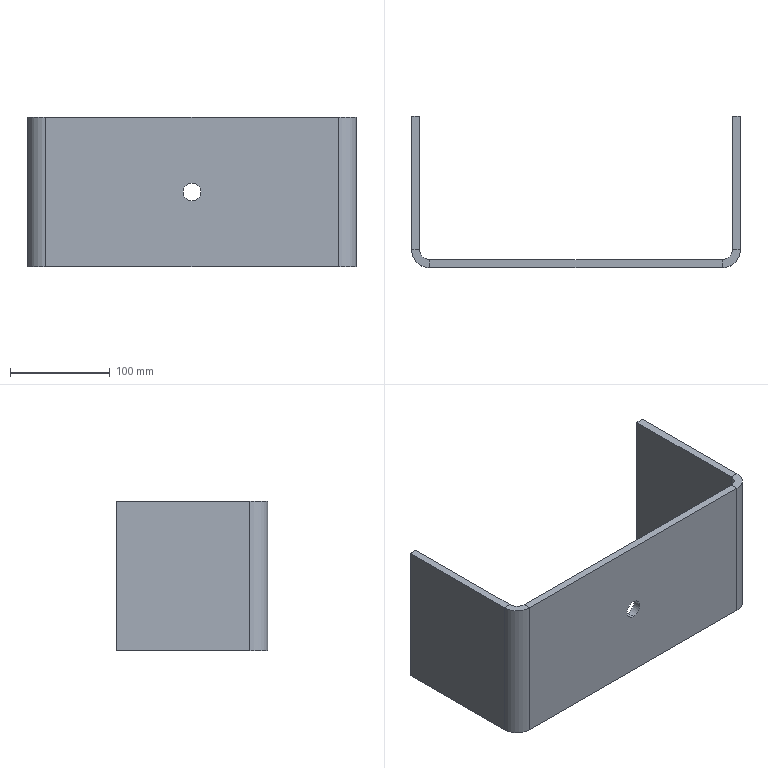Part | STEP file | A_SYL0380DJ1008_1_4-1_CHACHE_AS | 1 solid | 24 faces | box 330 x 152 x 150 mm | volume 725143 mm3 | plane 18 | cylinder 6 | commonest cylinder face diameters 18 x2 20 x2 36 x2
STEP:
#1=CARTESIAN_POINT('',(-165.,-62.,-75.));
#2=VERTEX_POINT('',#1);
#3=CARTESIAN_POINT('',(-165.,72.,-75.));
#4=VERTEX_POINT('',#3);
#5=CARTESIAN_POINT('',(-165.,-62.,-75.));
#6=DIRECTION('',(0.,1.,0.));
#7=VECTOR('',#6,1000.);
#8=LINE('',#5,#7);
#9=EDGE_CURVE('',#2,#4,#8,.T.);
#10=ORIENTED_EDGE('',*,*,#9,.F.);
#11=CARTESIAN_POINT('',(-165.,-62.,75.));
#12=VERTEX_POINT('',#11);
#13=CARTESIAN_POINT('',(-165.,-62.,75.));
#14=DIRECTION('',(0.,0.,-1.));
#15=VECTOR('',#14,1000.);
#16=LINE('',#13,#15);
#17=EDGE_CURVE('',#12,#2,#16,.T.);
#18=ORIENTED_EDGE('',*,*,#17,.F.);
#19=CARTESIAN_POINT('',(-165.,72.,75.));
#20=VERTEX_POINT('',#19);
#21=CARTESIAN_POINT('',(-165.,-62.,75.));
#22=DIRECTION('',(0.,1.,0.));
#23=VECTOR('',#22,1000.);
#24=LINE('',#21,#23);
#25=EDGE_CURVE('',#12,#20,#24,.T.);
#26=ORIENTED_EDGE('',*,*,#25,.T.);
#27=CARTESIAN_POINT('',(-165.,72.,75.));
#28=DIRECTION('',(0.,0.,-1.));
#29=VECTOR('',#28,1000.);
#30=LINE('',#27,#29);
#31=EDGE_CURVE('',#20,#4,#30,.T.);
#32=ORIENTED_EDGE('',*,*,#31,.T.);
#33=EDGE_LOOP('',(#10,#18,#26,#32));
#34=FACE_OUTER_BOUND('',#33,.T.);
#35=CARTESIAN_POINT('',(-165.,72.,-75.));
#36=DIRECTION('',(-1.,0.,0.));
#37=DIRECTION('',(0.,0.,1.));
#38=AXIS2_PLACEMENT_3D('',#35,#36,#37);
#39=PLANE('',#38);
#40=ADVANCED_FACE('',(#34),#39,.T.);
#41=CARTESIAN_POINT('',(165.,72.,75.));
#42=VERTEX_POINT('',#41);
#43=CARTESIAN_POINT('',(165.,-62.,75.));
#44=VERTEX_POINT('',#43);
#45=CARTESIAN_POINT('',(165.,72.,75.));
#46=DIRECTION('',(0.,-1.,0.));
#47=VECTOR('',#46,1000.);
#48=LINE('',#45,#47);
#49=EDGE_CURVE('',#42,#44,#48,.T.);
#50=ORIENTED_EDGE('',*,*,#49,.T.);
#51=CARTESIAN_POINT('',(165.,-62.,-75.));
#52=VERTEX_POINT('',#51);
#53=CARTESIAN_POINT('',(165.,-62.,-75.));
#54=DIRECTION('',(0.,0.,1.));
#55=VECTOR('',#54,1000.);
#56=LINE('',#53,#55);
#57=EDGE_CURVE('',#52,#44,#56,.T.);
#58=ORIENTED_EDGE('',*,*,#57,.F.);
#59=CARTESIAN_POINT('',(165.,72.,-75.));
#60=VERTEX_POINT('',#59);
#61=CARTESIAN_POINT('',(165.,72.,-75.));
#62=DIRECTION('',(0.,-1.,0.));
#63=VECTOR('',#62,1000.);
#64=LINE('',#61,#63);
#65=EDGE_CURVE('',#60,#52,#64,.T.);
#66=ORIENTED_EDGE('',*,*,#65,.F.);
#67=CARTESIAN_POINT('',(165.,72.,75.));
#68=DIRECTION('',(0.,0.,-1.));
#69=VECTOR('',#68,1000.);
#70=LINE('',#67,#69);
#71=EDGE_CURVE('',#42,#60,#70,.T.);
#72=ORIENTED_EDGE('',*,*,#71,.F.);
#73=EDGE_LOOP('',(#50,#58,#66,#72));
#74=FACE_OUTER_BOUND('',#73,.T.);
#75=CARTESIAN_POINT('',(165.,-80.,-75.));
#76=DIRECTION('',(1.,0.,0.));
#77=DIRECTION('',(0.,1.,0.));
#78=AXIS2_PLACEMENT_3D('',#75,#76,#77);
#79=PLANE('',#78);
#80=ADVANCED_FACE('',(#74),#79,.T.);
#81=CARTESIAN_POINT('',(147.,-80.,75.));
#82=VERTEX_POINT('',#81);
#83=CARTESIAN_POINT('',(147.,-62.,75.));
#84=DIRECTION('',(0.,0.,1.));
#85=DIRECTION('',(0.,-1.,0.));
#86=AXIS2_PLACEMENT_3D('',#83,#84,#85);
#87=CIRCLE('',#86,18.);
#88=EDGE_CURVE('',#82,#44,#87,.T.);
#89=ORIENTED_EDGE('',*,*,#88,.F.);
#90=CARTESIAN_POINT('',(147.,-80.,-75.));
#91=VERTEX_POINT('',#90);
#92=CARTESIAN_POINT('',(147.,-80.,75.));
#93=DIRECTION('',(0.,0.,-1.));
#94=VECTOR('',#93,1000.);
#95=LINE('',#92,#94);
#96=EDGE_CURVE('',#82,#91,#95,.T.);
#97=ORIENTED_EDGE('',*,*,#96,.T.);
#98=CARTESIAN_POINT('',(147.,-62.,-75.));
#99=DIRECTION('',(0.,0.,-1.));
#100=DIRECTION('',(1.,0.,0.));
#101=AXIS2_PLACEMENT_3D('',#98,#99,#100);
#102=CIRCLE('',#101,18.);
#103=EDGE_CURVE('',#52,#91,#102,.T.);
#104=ORIENTED_EDGE('',*,*,#103,.F.);
#105=ORIENTED_EDGE('',*,*,#57,.T.);
#106=EDGE_LOOP('',(#89,#97,#104,#105));
#107=FACE_OUTER_BOUND('',#106,.T.);
#108=CARTESIAN_POINT('',(147.,-62.,416.165));
#109=DIRECTION('',(0.,0.,-1.));
#110=DIRECTION('',(-1.,0.,0.));
#111=AXIS2_PLACEMENT_3D('',#108,#109,#110);
#112=CYLINDRICAL_SURFACE('',#111,18.);
#113=ADVANCED_FACE('',(#107),#112,.T.);
#114=CARTESIAN_POINT('',(0.,-80.,9.));
#115=VERTEX_POINT('',#114);
#116=CARTESIAN_POINT('',(0.,-72.,9.));
#117=VERTEX_POINT('',#116);
#118=CARTESIAN_POINT('',(0.,-80.,9.));
#119=DIRECTION('',(0.,1.,0.));
#120=VECTOR('',#119,1000.);
#121=LINE('',#118,#120);
#122=EDGE_CURVE('',#115,#117,#121,.T.);
#123=ORIENTED_EDGE('',*,*,#122,.F.);
#124=CARTESIAN_POINT('',(0.,-80.,-9.));
#125=VERTEX_POINT('',#124);
#126=CARTESIAN_POINT('',(0.,-80.,0.));
#127=DIRECTION('',(0.,1.,0.));
#128=DIRECTION('',(0.,0.,-1.));
#129=AXIS2_PLACEMENT_3D('',#126,#127,#128);
#130=CIRCLE('',#129,9.);
#131=EDGE_CURVE('',#125,#115,#130,.T.);
#132=ORIENTED_EDGE('',*,*,#131,.F.);
#133=CARTESIAN_POINT('',(0.,-72.,-9.));
#134=VERTEX_POINT('',#133);
#135=CARTESIAN_POINT('',(0.,-80.,-9.));
#136=DIRECTION('',(0.,1.,0.));
#137=VECTOR('',#136,1000.);
#138=LINE('',#135,#137);
#139=EDGE_CURVE('',#125,#134,#138,.T.);
#140=ORIENTED_EDGE('',*,*,#139,.T.);
#141=CARTESIAN_POINT('',(0.,-72.,0.));
#142=DIRECTION('',(0.,-1.,0.));
#143=DIRECTION('',(0.,0.,1.));
#144=AXIS2_PLACEMENT_3D('',#141,#142,#143);
#145=CIRCLE('',#144,9.);
#146=EDGE_CURVE('',#117,#134,#145,.T.);
#147=ORIENTED_EDGE('',*,*,#146,.F.);
#148=EDGE_LOOP('',(#123,#132,#140,#147));
#149=FACE_OUTER_BOUND('',#148,.T.);
#150=CARTESIAN_POINT('',(0.,-72.,0.));
#151=DIRECTION('',(0.,-1.,0.));
#152=DIRECTION('',(0.,0.,-1.));
#153=AXIS2_PLACEMENT_3D('',#150,#151,#152);
#154=CYLINDRICAL_SURFACE('',#153,9.);
#155=ADVANCED_FACE('',(#149),#154,.F.);
#156=CARTESIAN_POINT('',(0.,-72.,0.));
#157=DIRECTION('',(0.,-1.,0.));
#158=DIRECTION('',(0.,0.,-1.));
#159=AXIS2_PLACEMENT_3D('',#156,#157,#158);
#160=CIRCLE('',#159,9.);
#161=EDGE_CURVE('',#134,#117,#160,.T.);
#162=ORIENTED_EDGE('',*,*,#161,.F.);
#163=ORIENTED_EDGE('',*,*,#139,.F.);
#164=CARTESIAN_POINT('',(0.,-80.,0.));
#165=DIRECTION('',(0.,1.,0.));
#166=DIRECTION('',(0.,0.,1.));
#167=AXIS2_PLACEMENT_3D('',#164,#165,#166);
#168=CIRCLE('',#167,9.);
#169=EDGE_CURVE('',#115,#125,#168,.T.);
#170=ORIENTED_EDGE('',*,*,#169,.F.);
#171=ORIENTED_EDGE('',*,*,#122,.T.);
#172=EDGE_LOOP('',(#162,#163,#170,#171));
#173=FACE_OUTER_BOUND('',#172,.T.);
#174=CARTESIAN_POINT('',(0.,-72.,0.));
#175=DIRECTION('',(0.,-1.,0.));
#176=DIRECTION('',(0.,0.,-1.));
#177=AXIS2_PLACEMENT_3D('',#174,#175,#176);
#178=CYLINDRICAL_SURFACE('',#177,9.);
#179=ADVANCED_FACE('',(#173),#178,.F.);
#180=CARTESIAN_POINT('',(-157.,-62.,75.));
#181=VERTEX_POINT('',#180);
#182=CARTESIAN_POINT('',(-157.,72.,75.));
#183=VERTEX_POINT('',#182);
#184=CARTESIAN_POINT('',(-157.,-62.,75.));
#185=DIRECTION('',(0.,1.,0.));
#186=VECTOR('',#185,1000.);
#187=LINE('',#184,#186);
#188=EDGE_CURVE('',#181,#183,#187,.T.);
#189=ORIENTED_EDGE('',*,*,#188,.F.);
#190=CARTESIAN_POINT('',(-157.,-62.,-75.));
#191=VERTEX_POINT('',#190);
#192=CARTESIAN_POINT('',(-157.,-62.,-75.));
#193=DIRECTION('',(0.,0.,1.));
#194=VECTOR('',#193,1000.);
#195=LINE('',#192,#194);
#196=EDGE_CURVE('',#191,#181,#195,.T.);
#197=ORIENTED_EDGE('',*,*,#196,.F.);
#198=CARTESIAN_POINT('',(-157.,72.,-75.));
#199=VERTEX_POINT('',#198);
#200=CARTESIAN_POINT('',(-157.,-62.,-75.));
#201=DIRECTION('',(0.,1.,0.));
#202=VECTOR('',#201,1000.);
#203=LINE('',#200,#202);
#204=EDGE_CURVE('',#191,#199,#203,.T.);
#205=ORIENTED_EDGE('',*,*,#204,.T.);
#206=CARTESIAN_POINT('',(-157.,72.,75.));
#207=DIRECTION('',(0.,0.,-1.));
#208=VECTOR('',#207,1000.);
#209=LINE('',#206,#208);
#210=EDGE_CURVE('',#183,#199,#209,.T.);
#211=ORIENTED_EDGE('',*,*,#210,.F.);
#212=EDGE_LOOP('',(#189,#197,#205,#211));
#213=FACE_OUTER_BOUND('',#212,.T.);
#214=CARTESIAN_POINT('',(-157.,72.,-75.));
#215=DIRECTION('',(-1.,0.,0.));
#216=DIRECTION('',(0.,0.,1.));
#217=AXIS2_PLACEMENT_3D('',#214,#215,#216);
#218=PLANE('',#217);
#219=ADVANCED_FACE('',(#213),#218,.F.);
#220=CARTESIAN_POINT('',(-147.,-72.,-75.));
#221=VERTEX_POINT('',#220);
#222=CARTESIAN_POINT('',(-147.,-62.,-75.));
#223=DIRECTION('',(0.,0.,1.));
#224=DIRECTION('',(-1.,0.,0.));
#225=AXIS2_PLACEMENT_3D('',#222,#223,#224);
#226=CIRCLE('',#225,10.);
#227=EDGE_CURVE('',#191,#221,#226,.T.);
#228=ORIENTED_EDGE('',*,*,#227,.F.);
#229=ORIENTED_EDGE('',*,*,#196,.T.);
#230=CARTESIAN_POINT('',(-147.,-72.,75.));
#231=VERTEX_POINT('',#230);
#232=CARTESIAN_POINT('',(-147.,-62.,75.));
#233=DIRECTION('',(0.,0.,-1.));
#234=DIRECTION('',(0.,-1.,0.));
#235=AXIS2_PLACEMENT_3D('',#232,#233,#234);
#236=CIRCLE('',#235,10.);
#237=EDGE_CURVE('',#231,#181,#236,.T.);
#238=ORIENTED_EDGE('',*,*,#237,.F.);
#239=CARTESIAN_POINT('',(-147.,-72.,75.));
#240=DIRECTION('',(0.,0.,-1.));
#241=VECTOR('',#240,1000.);
#242=LINE('',#239,#241);
#243=EDGE_CURVE('',#231,#221,#242,.T.);
#244=ORIENTED_EDGE('',*,*,#243,.T.);
#245=EDGE_LOOP('',(#228,#229,#238,#244));
#246=FACE_OUTER_BOUND('',#245,.T.);
#247=CARTESIAN_POINT('',(-147.,-62.,416.165));
#248=DIRECTION('',(0.,0.,-1.));
#249=DIRECTION('',(-1.,0.,0.));
#250=AXIS2_PLACEMENT_3D('',#247,#248,#249);
#251=CYLINDRICAL_SURFACE('',#250,10.);
#252=ADVANCED_FACE('',(#246),#251,.F.);
#253=ORIENTED_EDGE('',*,*,#146,.T.);
#254=ORIENTED_EDGE('',*,*,#161,.T.);
#255=EDGE_LOOP('',(#253,#254));
#256=FACE_BOUND('',#255,.T.);
#257=CARTESIAN_POINT('',(147.,-72.,75.));
#258=VERTEX_POINT('',#257);
#259=CARTESIAN_POINT('',(147.,-72.,75.));
#260=DIRECTION('',(-1.,0.,0.));
#261=VECTOR('',#260,1000.);
#262=LINE('',#259,#261);
#263=EDGE_CURVE('',#258,#231,#262,.T.);
#264=ORIENTED_EDGE('',*,*,#263,.F.);
#265=CARTESIAN_POINT('',(147.,-72.,-75.));
#266=VERTEX_POINT('',#265);
#267=CARTESIAN_POINT('',(147.,-72.,-75.));
#268=DIRECTION('',(0.,0.,1.));
#269=VECTOR('',#268,1000.);
#270=LINE('',#267,#269);
#271=EDGE_CURVE('',#266,#258,#270,.T.);
#272=ORIENTED_EDGE('',*,*,#271,.F.);
#273=CARTESIAN_POINT('',(147.,-72.,-75.));
#274=DIRECTION('',(-1.,0.,0.));
#275=VECTOR('',#274,1000.);
#276=LINE('',#273,#275);
#277=EDGE_CURVE('',#266,#221,#276,.T.);
#278=ORIENTED_EDGE('',*,*,#277,.T.);
#279=ORIENTED_EDGE('',*,*,#243,.F.);
#280=EDGE_LOOP('',(#264,#272,#278,#279));
#281=FACE_OUTER_BOUND('',#280,.T.);
#282=CARTESIAN_POINT('',(-165.,-72.,-75.));
#283=DIRECTION('',(0.,-1.,0.));
#284=DIRECTION('',(0.,0.,-1.));
#285=AXIS2_PLACEMENT_3D('',#282,#283,#284);
#286=PLANE('',#285);
#287=ADVANCED_FACE('',(#256,#281),#286,.F.);
#288=CARTESIAN_POINT('',(157.,72.,-75.));
#289=VERTEX_POINT('',#288);
#290=CARTESIAN_POINT('',(157.,-62.,-75.));
#291=VERTEX_POINT('',#290);
#292=CARTESIAN_POINT('',(157.,72.,-75.));
#293=DIRECTION('',(0.,-1.,0.));
#294=VECTOR('',#293,1000.);
#295=LINE('',#292,#294);
#296=EDGE_CURVE('',#289,#291,#295,.T.);
#297=ORIENTED_EDGE('',*,*,#296,.T.);
#298=CARTESIAN_POINT('',(157.,-62.,75.));
#299=VERTEX_POINT('',#298);
#300=CARTESIAN_POINT('',(157.,-62.,75.));
#301=DIRECTION('',(0.,0.,-1.));
#302=VECTOR('',#301,1000.);
#303=LINE('',#300,#302);
#304=EDGE_CURVE('',#299,#291,#303,.T.);
#305=ORIENTED_EDGE('',*,*,#304,.F.);
#306=CARTESIAN_POINT('',(157.,72.,75.));
#307=VERTEX_POINT('',#306);
#308=CARTESIAN_POINT('',(157.,72.,75.));
#309=DIRECTION('',(0.,-1.,0.));
#310=VECTOR('',#309,1000.);
#311=LINE('',#308,#310);
#312=EDGE_CURVE('',#307,#299,#311,.T.);
#313=ORIENTED_EDGE('',*,*,#312,.F.);
#314=CARTESIAN_POINT('',(157.,72.,75.));
#315=DIRECTION('',(0.,0.,-1.));
#316=VECTOR('',#315,1000.);
#317=LINE('',#314,#316);
#318=EDGE_CURVE('',#307,#289,#317,.T.);
#319=ORIENTED_EDGE('',*,*,#318,.T.);
#320=EDGE_LOOP('',(#297,#305,#313,#319));
#321=FACE_OUTER_BOUND('',#320,.T.);
#322=CARTESIAN_POINT('',(157.,-80.,-75.));
#323=DIRECTION('',(1.,0.,0.));
#324=DIRECTION('',(0.,1.,0.));
#325=AXIS2_PLACEMENT_3D('',#322,#323,#324);
#326=PLANE('',#325);
#327=ADVANCED_FACE('',(#321),#326,.F.);
#328=CARTESIAN_POINT('',(147.,-62.,-75.));
#329=DIRECTION('',(0.,0.,1.));
#330=DIRECTION('',(0.,-1.,0.));
#331=AXIS2_PLACEMENT_3D('',#328,#329,#330);
#332=CIRCLE('',#331,10.);
#333=EDGE_CURVE('',#266,#291,#332,.T.);
#334=ORIENTED_EDGE('',*,*,#333,.F.);
#335=ORIENTED_EDGE('',*,*,#271,.T.);
#336=CARTESIAN_POINT('',(147.,-62.,75.));
#337=DIRECTION('',(0.,0.,-1.));
#338=DIRECTION('',(1.,0.,0.));
#339=AXIS2_PLACEMENT_3D('',#336,#337,#338);
#340=CIRCLE('',#339,10.);
#341=EDGE_CURVE('',#299,#258,#340,.T.);
#342=ORIENTED_EDGE('',*,*,#341,.F.);
#343=ORIENTED_EDGE('',*,*,#304,.T.);
#344=EDGE_LOOP('',(#334,#335,#342,#343));
#345=FACE_OUTER_BOUND('',#344,.T.);
#346=CARTESIAN_POINT('',(147.,-62.,416.165));
#347=DIRECTION('',(0.,0.,-1.));
#348=DIRECTION('',(-1.,0.,0.));
#349=AXIS2_PLACEMENT_3D('',#346,#347,#348);
#350=CYLINDRICAL_SURFACE('',#349,10.);
#351=ADVANCED_FACE('',(#345),#350,.F.);
#352=ORIENTED_EDGE('',*,*,#88,.T.);
#353=CARTESIAN_POINT('',(157.,-62.,75.));
#354=DIRECTION('',(1.,0.,0.));
#355=VECTOR('',#354,1000.);
#356=LINE('',#353,#355);
#357=EDGE_CURVE('',#299,#44,#356,.T.);
#358=ORIENTED_EDGE('',*,*,#357,.F.);
#359=ORIENTED_EDGE('',*,*,#341,.T.);
#360=CARTESIAN_POINT('',(147.,-72.,75.));
#361=DIRECTION('',(0.,-1.,0.));
#362=VECTOR('',#361,1000.);
#363=LINE('',#360,#362);
#364=EDGE_CURVE('',#258,#82,#363,.T.);
#365=ORIENTED_EDGE('',*,*,#364,.T.);
#366=EDGE_LOOP('',(#352,#358,#359,#365));
#367=FACE_OUTER_BOUND('',#366,.T.);
#368=CARTESIAN_POINT('',(147.,-62.,75.));
#369=DIRECTION('',(0.,0.,1.));
#370=DIRECTION('',(1.,0.,0.));
#371=AXIS2_PLACEMENT_3D('',#368,#369,#370);
#372=PLANE('',#371);
#373=ADVANCED_FACE('',(#367),#372,.T.);
#374=ORIENTED_EDGE('',*,*,#49,.F.);
#375=CARTESIAN_POINT('',(157.,72.,75.));
#376=DIRECTION('',(1.,0.,0.));
#377=VECTOR('',#376,1000.);
#378=LINE('',#375,#377);
#379=EDGE_CURVE('',#307,#42,#378,.T.);
#380=ORIENTED_EDGE('',*,*,#379,.F.);
#381=ORIENTED_EDGE('',*,*,#312,.T.);
#382=ORIENTED_EDGE('',*,*,#357,.T.);
#383=EDGE_LOOP('',(#374,#380,#381,#382));
#384=FACE_OUTER_BOUND('',#383,.T.);
#385=CARTESIAN_POINT('',(157.,-2.,75.));
#386=DIRECTION('',(0.,0.,-1.));
#387=DIRECTION('',(0.,-1.,0.));
#388=AXIS2_PLACEMENT_3D('',#385,#386,#387);
#389=PLANE('',#388);
#390=ADVANCED_FACE('',(#384),#389,.F.);
#391=ORIENTED_EDGE('',*,*,#71,.T.);
#392=CARTESIAN_POINT('',(157.,72.,-75.));
#393=DIRECTION('',(1.,0.,0.));
#394=VECTOR('',#393,1000.);
#395=LINE('',#392,#394);
#396=EDGE_CURVE('',#289,#60,#395,.T.);
#397=ORIENTED_EDGE('',*,*,#396,.F.);
#398=ORIENTED_EDGE('',*,*,#318,.F.);
#399=ORIENTED_EDGE('',*,*,#379,.T.);
#400=EDGE_LOOP('',(#391,#397,#398,#399));
#401=FACE_OUTER_BOUND('',#400,.T.);
#402=CARTESIAN_POINT('',(157.,72.,0.));
#403=DIRECTION('',(0.,1.,0.));
#404=DIRECTION('',(1.,0.,0.));
#405=AXIS2_PLACEMENT_3D('',#402,#403,#404);
#406=PLANE('',#405);
#407=ADVANCED_FACE('',(#401),#406,.T.);
#408=ORIENTED_EDGE('',*,*,#65,.T.);
#409=CARTESIAN_POINT('',(157.,-62.,-75.));
#410=DIRECTION('',(1.,0.,0.));
#411=VECTOR('',#410,1000.);
#412=LINE('',#409,#411);
#413=EDGE_CURVE('',#291,#52,#412,.T.);
#414=ORIENTED_EDGE('',*,*,#413,.F.);
#415=ORIENTED_EDGE('',*,*,#296,.F.);
#416=ORIENTED_EDGE('',*,*,#396,.T.);
#417=EDGE_LOOP('',(#408,#414,#415,#416));
#418=FACE_OUTER_BOUND('',#417,.T.);
#419=CARTESIAN_POINT('',(157.,-2.,-75.));
#420=DIRECTION('',(0.,0.,-1.));
#421=DIRECTION('',(0.,-1.,0.));
#422=AXIS2_PLACEMENT_3D('',#419,#420,#421);
#423=PLANE('',#422);
#424=ADVANCED_FACE('',(#418),#423,.T.);
#425=ORIENTED_EDGE('',*,*,#103,.T.);
#426=CARTESIAN_POINT('',(147.,-72.,-75.));
#427=DIRECTION('',(0.,-1.,0.));
#428=VECTOR('',#427,1000.);
#429=LINE('',#426,#428);
#430=EDGE_CURVE('',#266,#91,#429,.T.);
#431=ORIENTED_EDGE('',*,*,#430,.F.);
#432=ORIENTED_EDGE('',*,*,#333,.T.);
#433=ORIENTED_EDGE('',*,*,#413,.T.);
#434=EDGE_LOOP('',(#425,#431,#432,#433));
#435=FACE_OUTER_BOUND('',#434,.T.);
#436=CARTESIAN_POINT('',(147.,-62.,-75.));
#437=DIRECTION('',(0.,0.,1.));
#438=DIRECTION('',(1.,0.,0.));
#439=AXIS2_PLACEMENT_3D('',#436,#437,#438);
#440=PLANE('',#439);
#441=ADVANCED_FACE('',(#435),#440,.F.);
#442=CARTESIAN_POINT('',(-147.,-80.,-75.));
#443=VERTEX_POINT('',#442);
#444=CARTESIAN_POINT('',(-147.,-72.,-75.));
#445=DIRECTION('',(0.,-1.,0.));
#446=VECTOR('',#445,1000.);
#447=LINE('',#444,#446);
#448=EDGE_CURVE('',#221,#443,#447,.T.);
#449=ORIENTED_EDGE('',*,*,#448,.F.);
#450=ORIENTED_EDGE('',*,*,#277,.F.);
#451=ORIENTED_EDGE('',*,*,#430,.T.);
#452=CARTESIAN_POINT('',(147.,-80.,-75.));
#453=DIRECTION('',(-1.,0.,0.));
#454=VECTOR('',#453,1000.);
#455=LINE('',#452,#454);
#456=EDGE_CURVE('',#91,#443,#455,.T.);
#457=ORIENTED_EDGE('',*,*,#456,.T.);
#458=EDGE_LOOP('',(#449,#450,#451,#457));
#459=FACE_OUTER_BOUND('',#458,.T.);
#460=CARTESIAN_POINT('',(0.,-72.,-75.));
#461=DIRECTION('',(0.,0.,1.));
#462=DIRECTION('',(1.,0.,0.));
#463=AXIS2_PLACEMENT_3D('',#460,#461,#462);
#464=PLANE('',#463);
#465=ADVANCED_FACE('',(#459),#464,.F.);
#466=CARTESIAN_POINT('',(-147.,-62.,-75.));
#467=DIRECTION('',(0.,0.,-1.));
#468=DIRECTION('',(0.,-1.,0.));
#469=AXIS2_PLACEMENT_3D('',#466,#467,#468);
#470=CIRCLE('',#469,18.);
#471=EDGE_CURVE('',#443,#2,#470,.T.);
#472=ORIENTED_EDGE('',*,*,#471,.T.);
#473=CARTESIAN_POINT('',(-157.,-62.,-75.));
#474=DIRECTION('',(-1.,0.,0.));
#475=VECTOR('',#474,1000.);
#476=LINE('',#473,#475);
#477=EDGE_CURVE('',#191,#2,#476,.T.);
#478=ORIENTED_EDGE('',*,*,#477,.F.);
#479=ORIENTED_EDGE('',*,*,#227,.T.);
#480=ORIENTED_EDGE('',*,*,#448,.T.);
#481=EDGE_LOOP('',(#472,#478,#479,#480));
#482=FACE_OUTER_BOUND('',#481,.T.);
#483=CARTESIAN_POINT('',(-147.,-62.,-75.));
#484=DIRECTION('',(0.,0.,1.));
#485=DIRECTION('',(1.,0.,0.));
#486=AXIS2_PLACEMENT_3D('',#483,#484,#485);
#487=PLANE('',#486);
#488=ADVANCED_FACE('',(#482),#487,.F.);
#489=ORIENTED_EDGE('',*,*,#9,.T.);
#490=CARTESIAN_POINT('',(-157.,72.,-75.));
#491=DIRECTION('',(-1.,0.,0.));
#492=VECTOR('',#491,1000.);
#493=LINE('',#490,#492);
#494=EDGE_CURVE('',#199,#4,#493,.T.);
#495=ORIENTED_EDGE('',*,*,#494,.F.);
#496=ORIENTED_EDGE('',*,*,#204,.F.);
#497=ORIENTED_EDGE('',*,*,#477,.T.);
#498=EDGE_LOOP('',(#489,#495,#496,#497));
#499=FACE_OUTER_BOUND('',#498,.T.);
#500=CARTESIAN_POINT('',(-157.,-2.,-75.));
#501=DIRECTION('',(0.,0.,1.));
#502=DIRECTION('',(1.,0.,0.));
#503=AXIS2_PLACEMENT_3D('',#500,#501,#502);
#504=PLANE('',#503);
#505=ADVANCED_FACE('',(#499),#504,.F.);
#506=ORIENTED_EDGE('',*,*,#31,.F.);
#507=CARTESIAN_POINT('',(-157.,72.,75.));
#508=DIRECTION('',(-1.,0.,0.));
#509=VECTOR('',#508,1000.);
#510=LINE('',#507,#509);
#511=EDGE_CURVE('',#183,#20,#510,.T.);
#512=ORIENTED_EDGE('',*,*,#511,.F.);
#513=ORIENTED_EDGE('',*,*,#210,.T.);
#514=ORIENTED_EDGE('',*,*,#494,.T.);
#515=EDGE_LOOP('',(#506,#512,#513,#514));
#516=FACE_OUTER_BOUND('',#515,.T.);
#517=CARTESIAN_POINT('',(-157.,72.,0.));
#518=DIRECTION('',(0.,1.,0.));
#519=DIRECTION('',(1.,0.,0.));
#520=AXIS2_PLACEMENT_3D('',#517,#518,#519);
#521=PLANE('',#520);
#522=ADVANCED_FACE('',(#516),#521,.T.);
#523=ORIENTED_EDGE('',*,*,#25,.F.);
#524=CARTESIAN_POINT('',(-157.,-62.,75.));
#525=DIRECTION('',(-1.,0.,0.));
#526=VECTOR('',#525,1000.);
#527=LINE('',#524,#526);
#528=EDGE_CURVE('',#181,#12,#527,.T.);
#529=ORIENTED_EDGE('',*,*,#528,.F.);
#530=ORIENTED_EDGE('',*,*,#188,.T.);
#531=ORIENTED_EDGE('',*,*,#511,.T.);
#532=EDGE_LOOP('',(#523,#529,#530,#531));
#533=FACE_OUTER_BOUND('',#532,.T.);
#534=CARTESIAN_POINT('',(-157.,-2.,75.));
#535=DIRECTION('',(0.,0.,1.));
#536=DIRECTION('',(1.,0.,0.));
#537=AXIS2_PLACEMENT_3D('',#534,#535,#536);
#538=PLANE('',#537);
#539=ADVANCED_FACE('',(#533),#538,.T.);
#540=CARTESIAN_POINT('',(-147.,-80.,75.));
#541=VERTEX_POINT('',#540);
#542=CARTESIAN_POINT('',(-147.,-62.,75.));
#543=DIRECTION('',(0.,0.,1.));
#544=DIRECTION('',(-1.,0.,0.));
#545=AXIS2_PLACEMENT_3D('',#542,#543,#544);
#546=CIRCLE('',#545,18.);
#547=EDGE_CURVE('',#12,#541,#546,.T.);
#548=ORIENTED_EDGE('',*,*,#547,.T.);
#549=CARTESIAN_POINT('',(-147.,-72.,75.));
#550=DIRECTION('',(0.,-1.,0.));
#551=VECTOR('',#550,1000.);
#552=LINE('',#549,#551);
#553=EDGE_CURVE('',#231,#541,#552,.T.);
#554=ORIENTED_EDGE('',*,*,#553,.F.);
#555=ORIENTED_EDGE('',*,*,#237,.T.);
#556=ORIENTED_EDGE('',*,*,#528,.T.);
#557=EDGE_LOOP('',(#548,#554,#555,#556));
#558=FACE_OUTER_BOUND('',#557,.T.);
#559=CARTESIAN_POINT('',(-147.,-62.,75.));
#560=DIRECTION('',(0.,0.,1.));
#561=DIRECTION('',(1.,0.,0.));
#562=AXIS2_PLACEMENT_3D('',#559,#560,#561);
#563=PLANE('',#562);
#564=ADVANCED_FACE('',(#558),#563,.T.);
#565=CARTESIAN_POINT('',(147.,-80.,75.));
#566=DIRECTION('',(-1.,0.,0.));
#567=VECTOR('',#566,1000.);
#568=LINE('',#565,#567);
#569=EDGE_CURVE('',#82,#541,#568,.T.);
#570=ORIENTED_EDGE('',*,*,#569,.F.);
#571=ORIENTED_EDGE('',*,*,#364,.F.);
#572=ORIENTED_EDGE('',*,*,#263,.T.);
#573=ORIENTED_EDGE('',*,*,#553,.T.);
#574=EDGE_LOOP('',(#570,#571,#572,#573));
#575=FACE_OUTER_BOUND('',#574,.T.);
#576=CARTESIAN_POINT('',(0.,-72.,75.));
#577=DIRECTION('',(0.,0.,1.));
#578=DIRECTION('',(1.,0.,0.));
#579=AXIS2_PLACEMENT_3D('',#576,#577,#578);
#580=PLANE('',#579);
#581=ADVANCED_FACE('',(#575),#580,.T.);
#582=ORIENTED_EDGE('',*,*,#131,.T.);
#583=ORIENTED_EDGE('',*,*,#169,.T.);
#584=EDGE_LOOP('',(#582,#583));
#585=FACE_BOUND('',#584,.T.);
#586=ORIENTED_EDGE('',*,*,#456,.F.);
#587=ORIENTED_EDGE('',*,*,#96,.F.);
#588=ORIENTED_EDGE('',*,*,#569,.T.);
#589=CARTESIAN_POINT('',(-147.,-80.,-75.));
#590=DIRECTION('',(0.,0.,1.));
#591=VECTOR('',#590,1000.);
#592=LINE('',#589,#591);
#593=EDGE_CURVE('',#443,#541,#592,.T.);
#594=ORIENTED_EDGE('',*,*,#593,.F.);
#595=EDGE_LOOP('',(#586,#587,#588,#594));
#596=FACE_OUTER_BOUND('',#595,.T.);
#597=CARTESIAN_POINT('',(-165.,-80.,-75.));
#598=DIRECTION('',(0.,-1.,0.));
#599=DIRECTION('',(0.,0.,-1.));
#600=AXIS2_PLACEMENT_3D('',#597,#598,#599);
#601=PLANE('',#600);
#602=ADVANCED_FACE('',(#585,#596),#601,.T.);
#603=ORIENTED_EDGE('',*,*,#547,.F.);
#604=ORIENTED_EDGE('',*,*,#17,.T.);
#605=ORIENTED_EDGE('',*,*,#471,.F.);
#606=ORIENTED_EDGE('',*,*,#593,.T.);
#607=EDGE_LOOP('',(#603,#604,#605,#606));
#608=FACE_OUTER_BOUND('',#607,.T.);
#609=CARTESIAN_POINT('',(-147.,-62.,416.165));
#610=DIRECTION('',(0.,0.,-1.));
#611=DIRECTION('',(-1.,0.,0.));
#612=AXIS2_PLACEMENT_3D('',#609,#610,#611);
#613=CYLINDRICAL_SURFACE('',#612,18.);
#614=ADVANCED_FACE('',(#608),#613,.T.);
#615=CLOSED_SHELL('',(#40,#80,#113,#155,#179,#219,#252,#287,#327,#351,#373,#390,#407,#424,#441,#465,#488,#505,#522,#539,#564,#581,#602,#614));
#616=MANIFOLD_SOLID_BREP('',#615);
#617=CARTESIAN_POINT('',(0.,0.,0.));
#618=DIRECTION('',(0.,0.,1.));
#619=DIRECTION('',(1.,0.,0.));
#620=AXIS2_PLACEMENT_3D('',#617,#618,#619);
#621=(LENGTH_UNIT()NAMED_UNIT(*)SI_UNIT(.MILLI.,.METRE.));
#622=UNCERTAINTY_MEASURE_WITH_UNIT(LENGTH_MEASURE(0.00001),#621,'','');
#623=(NAMED_UNIT(*)PLANE_ANGLE_UNIT()SI_UNIT($,.RADIAN.));
#624=(NAMED_UNIT(*)SI_UNIT($,.STERADIAN.)SOLID_ANGLE_UNIT());
#625=(GEOMETRIC_REPRESENTATION_CONTEXT(3)GLOBAL_UNCERTAINTY_ASSIGNED_CONTEXT((#622))GLOBAL_UNIT_ASSIGNED_CONTEXT((#621,#623,#624))REPRESENTATION_CONTEXT('',''));
#626=ADVANCED_BREP_SHAPE_REPRESENTATION('',(#616,#620),#625);